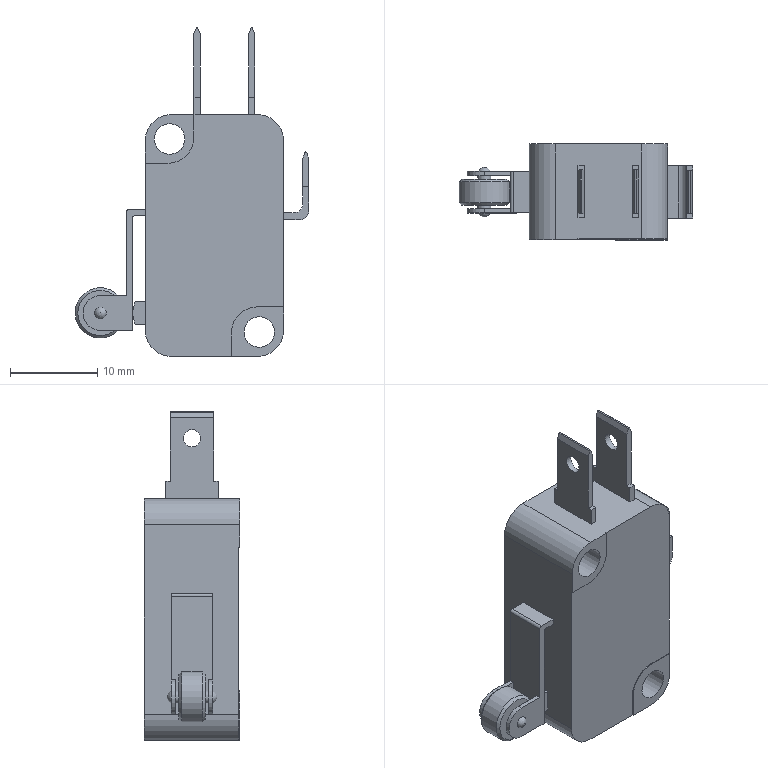Part | STEP file | E050000001 | 1 solid | 89 faces | box 26.859 x 11 x 37.801 mm | volume 4792 mm3 | plane 61 | cylinder 24 | sphere 2 | cone 2 | commonest cylinder face diameters 6 x6 2 x5 0.2 x3 0.6 x2 1.5 x2 3.5 x2